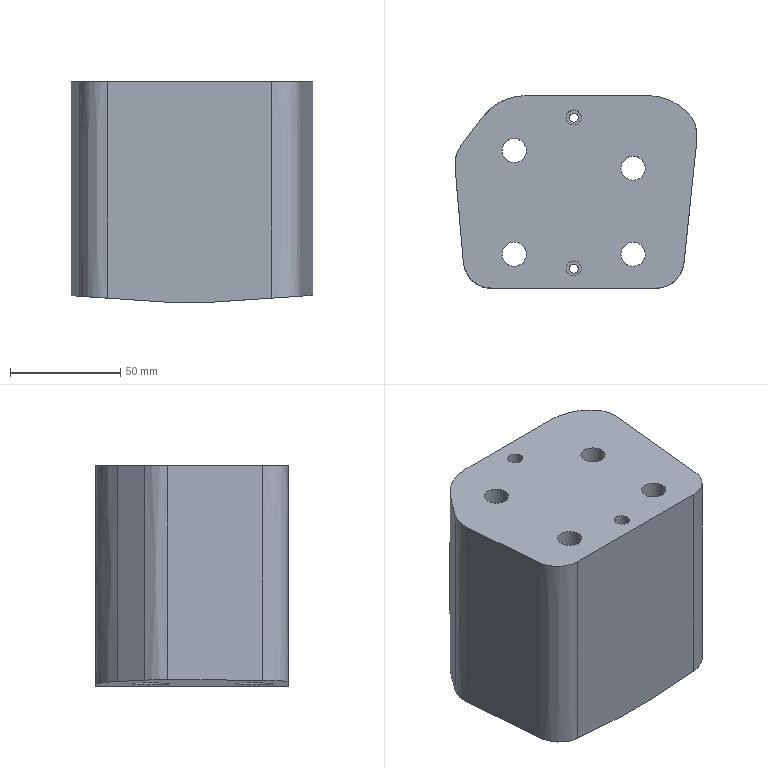Part | STEP file | lll_id3602_x_t | 1 solid | 42 faces | box 109.865 x 87.36 x 100 mm | volume 784681 mm3 | cylinder 18 | plane 18 | other 4 | cone 2 | commonest cylinder face diameters 11 x6 17 x4 4.1 x2 6.8 x2 8.506 x2 30 x1
STEP:
#1=CARTESIAN_POINT('',(3585.33,71.615,29.5));
#2=VERTEX_POINT('',#1);
#3=CARTESIAN_POINT('',(3587.38,71.615,29.5));
#4=DIRECTION('',(0.,0.,1.));
#5=DIRECTION('',(-1.,0.,0.));
#6=AXIS2_PLACEMENT_3D('',#3,#4,#5);
#7=CIRCLE('',#6,2.05);
#8=EDGE_CURVE('',#2,#2,#7,.T.);
#9=ORIENTED_EDGE('',*,*,#8,.T.);
#10=EDGE_LOOP('',(#9));
#11=FACE_BOUND('',#10,.T.);
#12=CARTESIAN_POINT('',(3587.38,73.665,-7.5));
#13=VERTEX_POINT('',#12);
#14=CARTESIAN_POINT('',(3587.38,71.615,-7.5));
#15=DIRECTION('',(0.,-0.000000008,1.));
#16=DIRECTION('',(0.,1.,0.000000008));
#17=AXIS2_PLACEMENT_3D('',#14,#15,#16);
#18=CIRCLE('',#17,2.05);
#19=EDGE_CURVE('',#13,#13,#18,.T.);
#20=ORIENTED_EDGE('',*,*,#19,.F.);
#21=EDGE_LOOP('',(#20));
#22=FACE_BOUND('',#21,.T.);
#23=CARTESIAN_POINT('',(3587.38,71.615,42.5));
#24=DIRECTION('',(0.,0.,-1.));
#25=DIRECTION('',(-0.0006834,1.,0.));
#26=AXIS2_PLACEMENT_3D('',#23,#24,#25);
#27=CYLINDRICAL_SURFACE('',#26,2.05);
#28=ADVANCED_FACE('',(#11,#22),#27,.F.);
#29=CARTESIAN_POINT('',(3585.326,140.05,29.5));
#30=VERTEX_POINT('',#29);
#31=CARTESIAN_POINT('',(3587.376,140.05,29.5));
#32=DIRECTION('',(0.,0.,1.));
#33=DIRECTION('',(-1.,0.,0.));
#34=AXIS2_PLACEMENT_3D('',#31,#32,#33);
#35=CIRCLE('',#34,2.05);
#36=EDGE_CURVE('',#30,#30,#35,.T.);
#37=ORIENTED_EDGE('',*,*,#36,.T.);
#38=EDGE_LOOP('',(#37));
#39=FACE_BOUND('',#38,.T.);
#40=CARTESIAN_POINT('',(3587.376,142.1,-7.5));
#41=VERTEX_POINT('',#40);
#42=CARTESIAN_POINT('',(3587.376,140.05,-7.5));
#43=DIRECTION('',(0.,-0.000000008,1.));
#44=DIRECTION('',(0.,1.,0.000000008));
#45=AXIS2_PLACEMENT_3D('',#42,#43,#44);
#46=CIRCLE('',#45,2.05);
#47=EDGE_CURVE('',#41,#41,#46,.T.);
#48=ORIENTED_EDGE('',*,*,#47,.F.);
#49=EDGE_LOOP('',(#48));
#50=FACE_BOUND('',#49,.T.);
#51=CARTESIAN_POINT('',(3587.376,140.05,42.5));
#52=DIRECTION('',(0.,0.,-1.));
#53=DIRECTION('',(0.,-1.,0.));
#54=AXIS2_PLACEMENT_3D('',#51,#52,#53);
#55=CYLINDRICAL_SURFACE('',#54,2.05);
#56=ADVANCED_FACE('',(#39,#50),#55,.F.);
#57=CARTESIAN_POINT('',(3614.279,69.531,62.5));
#58=VERTEX_POINT('',#57);
#59=CARTESIAN_POINT('',(3614.279,78.031,62.5));
#60=DIRECTION('',(0.,0.,-1.));
#61=DIRECTION('',(0.,-1.,0.));
#62=AXIS2_PLACEMENT_3D('',#59,#60,#61);
#63=CIRCLE('',#62,8.5);
#64=EDGE_CURVE('',#58,#58,#63,.T.);
#65=ORIENTED_EDGE('',*,*,#64,.F.);
#66=EDGE_LOOP('',(#65));
#67=FACE_BOUND('',#66,.T.);
#68=CARTESIAN_POINT('',(3622.779,78.031,-5.757));
#69=VERTEX_POINT('',#68);
#70=CARTESIAN_POINT('',(3614.279,78.031,-6.338));
#71=DIRECTION('',(0.06817,0.,-0.9977));
#72=DIRECTION('',(0.9977,0.,0.06817));
#73=AXIS2_PLACEMENT_3D('',#70,#71,#72);
#74=ELLIPSE('',#73,8.52,8.5);
#75=EDGE_CURVE('',#69,#69,#74,.T.);
#76=ORIENTED_EDGE('',*,*,#75,.T.);
#77=EDGE_LOOP('',(#76));
#78=FACE_BOUND('',#77,.T.);
#79=CARTESIAN_POINT('',(3614.279,78.031,12.5));
#80=DIRECTION('',(0.,0.,1.));
#81=DIRECTION('',(0.,1.,0.));
#82=AXIS2_PLACEMENT_3D('',#79,#80,#81);
#83=CYLINDRICAL_SURFACE('',#82,8.5);
#84=ADVANCED_FACE('',(#67,#78),#83,.F.);
#85=CARTESIAN_POINT('',(3638.507,142.694,92.5));
#86=VERTEX_POINT('',#85);
#87=CARTESIAN_POINT('',(3638.938,142.263,92.5));
#88=VERTEX_POINT('',#87);
#89=CARTESIAN_POINT('',(3565.868,215.334,92.5));
#90=DIRECTION('',(0.7071,-0.7071,0.));
#91=VECTOR('',#90,1.);
#92=LINE('',#89,#91);
#93=EDGE_CURVE('',#86,#88,#92,.T.);
#94=ORIENTED_EDGE('',*,*,#93,.T.);
#95=CARTESIAN_POINT('',(3638.938,142.263,-4.653));
#96=VERTEX_POINT('',#95);
#97=CARTESIAN_POINT('',(3638.938,142.263,0.00002208));
#98=DIRECTION('',(0.,0.000000008,-1.));
#99=VECTOR('',#98,1.);
#100=LINE('',#97,#99);
#101=EDGE_CURVE('',#88,#96,#100,.T.);
#102=ORIENTED_EDGE('',*,*,#101,.T.);
#103=CARTESIAN_POINT('',(3638.507,142.694,-4.682));
#104=VERTEX_POINT('',#103);
#105=CARTESIAN_POINT('',(3614.187,167.015,-6.344));
#106=DIRECTION('',(-0.7063,0.7063,-0.04826));
#107=VECTOR('',#106,1.);
#108=LINE('',#105,#107);
#109=EDGE_CURVE('',#96,#104,#108,.T.);
#110=ORIENTED_EDGE('',*,*,#109,.T.);
#111=CARTESIAN_POINT('',(3638.507,142.694,0.00002209));
#112=DIRECTION('',(0.,-0.000000008,1.));
#113=VECTOR('',#112,1.);
#114=LINE('',#111,#113);
#115=EDGE_CURVE('',#104,#86,#114,.T.);
#116=ORIENTED_EDGE('',*,*,#115,.T.);
#117=EDGE_LOOP('',(#94,#102,#110,#116));
#118=FACE_OUTER_BOUND('',#117,.T.);
#119=CARTESIAN_POINT('',(3638.507,142.694,0.00002209));
#120=DIRECTION('',(0.7071,0.7071,0.000000005));
#121=DIRECTION('',(0.7071,-0.7071,-0.000000005));
#122=AXIS2_PLACEMENT_3D('',#119,#120,#121);
#123=PLANE('',#122);
#124=ADVANCED_FACE('',(#118),#123,.T.);
#125=CARTESIAN_POINT('',(3577.268,62.657,-7.5));
#126=VERTEX_POINT('',#125);
#127=CARTESIAN_POINT('',(3550.037,62.657,-5.639));
#128=VERTEX_POINT('',#127);
#129=CARTESIAN_POINT('',(3586.78,62.657,-8.15));
#130=DIRECTION('',(-0.9977,-0.000000001,0.06817));
#131=VECTOR('',#130,1.);
#132=LINE('',#129,#131);
#133=EDGE_CURVE('',#126,#128,#132,.T.);
#134=ORIENTED_EDGE('',*,*,#133,.F.);
#135=CARTESIAN_POINT('',(3597.268,62.657,-7.5));
#136=VERTEX_POINT('',#135);
#137=CARTESIAN_POINT('',(3633.202,62.657,-7.5));
#138=DIRECTION('',(-1.,0.,0.));
#139=VECTOR('',#138,1.);
#140=LINE('',#137,#139);
#141=EDGE_CURVE('',#136,#126,#140,.T.);
#142=ORIENTED_EDGE('',*,*,#141,.F.);
#143=CARTESIAN_POINT('',(3624.637,62.657,-5.63));
#144=VERTEX_POINT('',#143);
#145=CARTESIAN_POINT('',(3597.268,62.657,-7.5));
#146=DIRECTION('',(-0.9977,0.,-0.06817));
#147=VECTOR('',#146,1.);
#148=LINE('',#145,#147);
#149=EDGE_CURVE('',#144,#136,#148,.T.);
#150=ORIENTED_EDGE('',*,*,#149,.F.);
#151=CARTESIAN_POINT('',(3624.637,62.657,92.5));
#152=VERTEX_POINT('',#151);
#153=CARTESIAN_POINT('',(3624.637,62.657,0.0000176));
#154=DIRECTION('',(0.,-0.000000008,1.));
#155=VECTOR('',#154,1.);
#156=LINE('',#153,#155);
#157=EDGE_CURVE('',#144,#152,#156,.T.);
#158=ORIENTED_EDGE('',*,*,#157,.T.);
#159=CARTESIAN_POINT('',(3550.037,62.657,92.5));
#160=VERTEX_POINT('',#159);
#161=CARTESIAN_POINT('',(3587.337,62.657,92.5));
#162=DIRECTION('',(-1.,0.,0.));
#163=VECTOR('',#162,1.);
#164=LINE('',#161,#163);
#165=EDGE_CURVE('',#152,#160,#164,.T.);
#166=ORIENTED_EDGE('',*,*,#165,.T.);
#167=CARTESIAN_POINT('',(3550.037,62.657,0.0000176));
#168=DIRECTION('',(0.,-0.000000008,1.));
#169=VECTOR('',#168,1.);
#170=LINE('',#167,#169);
#171=EDGE_CURVE('',#128,#160,#170,.T.);
#172=ORIENTED_EDGE('',*,*,#171,.F.);
#173=EDGE_LOOP('',(#134,#142,#150,#158,#166,#172));
#174=FACE_OUTER_BOUND('',#173,.T.);
#175=CARTESIAN_POINT('',(3587.337,62.657,0.0000176));
#176=DIRECTION('',(0.,1.,0.000000008));
#177=DIRECTION('',(-1.,0.,0.));
#178=AXIS2_PLACEMENT_3D('',#175,#176,#177);
#179=PLANE('',#178);
#180=ADVANCED_FACE('',(#174),#179,.F.);
#181=ORIENTED_EDGE('',*,*,#157,.F.);
#182=CARTESIAN_POINT('',(3637.367,74.119,-4.76));
#183=VERTEX_POINT('',#182);
#184=CARTESIAN_POINT('',(3624.637,62.657,-5.63));
#185=CARTESIAN_POINT('',(3627.788,62.657,-5.415));
#186=CARTESIAN_POINT('',(3630.864,63.843,-5.204));
#187=CARTESIAN_POINT('',(3635.521,68.029,-4.886));
#188=CARTESIAN_POINT('',(3637.037,70.974,-4.783));
#189=CARTESIAN_POINT('',(3637.367,74.119,-4.76));
#190=B_SPLINE_CURVE_WITH_KNOTS('',3,(#184,#185,#186,#187,#188,#189),.UNSPECIFIED.,.F.,.F.,(4,2,4),(0.,0.5,1.),.UNSPECIFIED.);
#191=EDGE_CURVE('',#144,#183,#190,.T.);
#192=ORIENTED_EDGE('',*,*,#191,.T.);
#193=CARTESIAN_POINT('',(3637.367,74.119,92.5));
#194=VERTEX_POINT('',#193);
#195=CARTESIAN_POINT('',(3637.367,74.119,0.00001769));
#196=DIRECTION('',(0.,-0.000000008,1.));
#197=VECTOR('',#196,1.);
#198=LINE('',#195,#197);
#199=EDGE_CURVE('',#183,#194,#198,.T.);
#200=ORIENTED_EDGE('',*,*,#199,.T.);
#201=CARTESIAN_POINT('',(3637.367,74.119,92.5));
#202=CARTESIAN_POINT('',(3637.037,70.982,92.5));
#203=CARTESIAN_POINT('',(3635.532,68.044,92.5));
#204=CARTESIAN_POINT('',(3630.881,63.852,92.5));
#205=CARTESIAN_POINT('',(3627.795,62.657,92.5));
#206=CARTESIAN_POINT('',(3624.637,62.657,92.5));
#207=B_SPLINE_CURVE_WITH_KNOTS('',3,(#201,#202,#203,#204,#205,#206),.UNSPECIFIED.,.F.,.F.,(4,2,4),(0.,0.5,1.),.UNSPECIFIED.);
#208=EDGE_CURVE('',#194,#152,#207,.T.);
#209=ORIENTED_EDGE('',*,*,#208,.T.);
#210=EDGE_LOOP('',(#181,#192,#200,#209));
#211=FACE_OUTER_BOUND('',#210,.T.);
#212=CARTESIAN_POINT('',(3637.367,74.119,0.00001769));
#213=CARTESIAN_POINT('',(3637.202,72.546,0.00001768));
#214=CARTESIAN_POINT('',(3636.76,71.054,0.00001767));
#215=CARTESIAN_POINT('',(3635.324,68.237,0.00001764));
#216=CARTESIAN_POINT('',(3634.377,67.002,0.00001763));
#217=CARTESIAN_POINT('',(3632.027,64.886,0.00001762));
#218=CARTESIAN_POINT('',(3630.701,64.074,0.00001761));
#219=CARTESIAN_POINT('',(3627.748,62.94,0.0000176));
#220=CARTESIAN_POINT('',(3626.219,62.657,0.0000176));
#221=CARTESIAN_POINT('',(3624.637,62.657,0.0000176));
#222=B_SPLINE_CURVE_WITH_KNOTS('',3,(#212,#213,#214,#215,#216,#217,#218,#219,#220,#221),.UNSPECIFIED.,.F.,.F.,(4,2,2,2,4),(0.,0.25,0.5,0.75,1.),.UNSPECIFIED.);
#223=DIRECTION('',(0.,-0.000000008,1.));
#224=VECTOR('',#223,1.);
#225=SURFACE_OF_LINEAR_EXTRUSION('',#222,#224);
#226=ADVANCED_FACE('',(#211),#225,.F.);
#227=CARTESIAN_POINT('',(3643.25,130.089,-4.358));
#228=VERTEX_POINT('',#227);
#229=CARTESIAN_POINT('',(3639.156,91.137,-4.638));
#230=DIRECTION('',(0.1045,0.9945,0.007142));
#231=VECTOR('',#230,1.);
#232=LINE('',#229,#231);
#233=EDGE_CURVE('',#183,#228,#232,.T.);
#234=ORIENTED_EDGE('',*,*,#233,.T.);
#235=CARTESIAN_POINT('',(3643.25,130.089,92.5));
#236=VERTEX_POINT('',#235);
#237=CARTESIAN_POINT('',(3643.25,130.089,0.00001811));
#238=DIRECTION('',(0.,-0.000000008,1.));
#239=VECTOR('',#238,1.);
#240=LINE('',#237,#239);
#241=EDGE_CURVE('',#228,#236,#240,.T.);
#242=ORIENTED_EDGE('',*,*,#241,.T.);
#243=CARTESIAN_POINT('',(3639.152,91.104,92.5));
#244=DIRECTION('',(-0.1045,-0.9945,0.));
#245=VECTOR('',#244,1.);
#246=LINE('',#243,#245);
#247=EDGE_CURVE('',#236,#194,#246,.T.);
#248=ORIENTED_EDGE('',*,*,#247,.T.);
#249=ORIENTED_EDGE('',*,*,#199,.F.);
#250=EDGE_LOOP('',(#234,#242,#248,#249));
#251=FACE_OUTER_BOUND('',#250,.T.);
#252=CARTESIAN_POINT('',(3639.152,91.104,0.00001782));
#253=DIRECTION('',(-0.9945,0.1045,0.000000001));
#254=DIRECTION('',(-0.1045,-0.9945,-0.000000008));
#255=AXIS2_PLACEMENT_3D('',#252,#253,#254);
#256=PLANE('',#255);
#257=ADVANCED_FACE('',(#251),#256,.F.);
#258=CARTESIAN_POINT('',(3614.279,108.531,62.5));
#259=VERTEX_POINT('',#258);
#260=CARTESIAN_POINT('',(3614.279,117.031,62.5));
#261=DIRECTION('',(0.,0.,-1.));
#262=DIRECTION('',(0.,-1.,0.));
#263=AXIS2_PLACEMENT_3D('',#260,#261,#262);
#264=CIRCLE('',#263,8.5);
#265=EDGE_CURVE('',#259,#259,#264,.T.);
#266=ORIENTED_EDGE('',*,*,#265,.F.);
#267=EDGE_LOOP('',(#266));
#268=FACE_BOUND('',#267,.T.);
#269=CARTESIAN_POINT('',(3622.779,117.031,-5.757));
#270=VERTEX_POINT('',#269);
#271=CARTESIAN_POINT('',(3614.279,117.031,-6.338));
#272=DIRECTION('',(-0.06817,0.,0.9977));
#273=DIRECTION('',(0.9977,0.,0.06817));
#274=AXIS2_PLACEMENT_3D('',#271,#272,#273);
#275=ELLIPSE('',#274,8.52,8.5);
#276=EDGE_CURVE('',#270,#270,#275,.T.);
#277=ORIENTED_EDGE('',*,*,#276,.F.);
#278=EDGE_LOOP('',(#277));
#279=FACE_BOUND('',#278,.T.);
#280=CARTESIAN_POINT('',(3614.279,117.031,12.5));
#281=DIRECTION('',(0.,0.,1.));
#282=DIRECTION('',(0.,1.,0.));
#283=AXIS2_PLACEMENT_3D('',#280,#281,#282);
#284=CYLINDRICAL_SURFACE('',#283,8.5);
#285=ADVANCED_FACE('',(#268,#279),#284,.F.);
#286=ORIENTED_EDGE('',*,*,#47,.T.);
#287=EDGE_LOOP('',(#286));
#288=FACE_BOUND('',#287,.T.);
#289=ORIENTED_EDGE('',*,*,#19,.T.);
#290=EDGE_LOOP('',(#289));
#291=FACE_BOUND('',#290,.T.);
#292=CARTESIAN_POINT('',(3587.38,92.115,-7.5));
#293=VERTEX_POINT('',#292);
#294=CARTESIAN_POINT('',(3587.38,86.615,-7.5));
#295=DIRECTION('',(0.,-0.000000008,1.));
#296=DIRECTION('',(0.,1.,0.000000008));
#297=AXIS2_PLACEMENT_3D('',#294,#295,#296);
#298=CIRCLE('',#297,5.5);
#299=EDGE_CURVE('',#293,#293,#298,.T.);
#300=ORIENTED_EDGE('',*,*,#299,.T.);
#301=EDGE_LOOP('',(#300));
#302=FACE_BOUND('',#301,.T.);
#303=CARTESIAN_POINT('',(3587.38,130.115,-7.5));
#304=VERTEX_POINT('',#303);
#305=CARTESIAN_POINT('',(3587.38,124.615,-7.5));
#306=DIRECTION('',(0.,-0.000000008,1.));
#307=DIRECTION('',(0.,1.,0.000000008));
#308=AXIS2_PLACEMENT_3D('',#305,#306,#307);
#309=CIRCLE('',#308,5.5);
#310=EDGE_CURVE('',#304,#304,#309,.T.);
#311=ORIENTED_EDGE('',*,*,#310,.T.);
#312=EDGE_LOOP('',(#311));
#313=FACE_BOUND('',#312,.T.);
#314=ORIENTED_EDGE('',*,*,#141,.T.);
#315=CARTESIAN_POINT('',(3577.268,150.017,-7.5));
#316=VERTEX_POINT('',#315);
#317=CARTESIAN_POINT('',(3577.268,65.944,-7.5));
#318=DIRECTION('',(-0.000000111,1.,0.000000008));
#319=VECTOR('',#318,1.);
#320=LINE('',#317,#319);
#321=EDGE_CURVE('',#126,#316,#320,.T.);
#322=ORIENTED_EDGE('',*,*,#321,.T.);
#323=CARTESIAN_POINT('',(3597.268,150.017,-7.5));
#324=VERTEX_POINT('',#323);
#325=CARTESIAN_POINT('',(3633.202,150.017,-7.5));
#326=DIRECTION('',(1.,0.,0.));
#327=VECTOR('',#326,1.);
#328=LINE('',#325,#327);
#329=EDGE_CURVE('',#316,#324,#328,.T.);
#330=ORIENTED_EDGE('',*,*,#329,.T.);
#331=CARTESIAN_POINT('',(3597.268,62.657,-7.5));
#332=DIRECTION('',(0.,1.,0.));
#333=VECTOR('',#332,1.);
#334=LINE('',#331,#333);
#335=EDGE_CURVE('',#136,#324,#334,.T.);
#336=ORIENTED_EDGE('',*,*,#335,.F.);
#337=EDGE_LOOP('',(#314,#322,#330,#336));
#338=FACE_BOUND('',#337,.T.);
#339=CARTESIAN_POINT('',(3633.202,65.944,-7.5));
#340=DIRECTION('',(0.,-0.000000008,1.));
#341=DIRECTION('',(0.,1.,0.000000008));
#342=AXIS2_PLACEMENT_3D('',#339,#340,#341);
#343=PLANE('',#342);
#344=ADVANCED_FACE('',(#288,#291,#302,#313,#338),#343,.F.);
#345=ORIENTED_EDGE('',*,*,#64,.T.);
#346=EDGE_LOOP('',(#345));
#347=FACE_BOUND('',#346,.T.);
#348=CARTESIAN_POINT('',(3608.779,78.031,62.5));
#349=VERTEX_POINT('',#348);
#350=CARTESIAN_POINT('',(3614.279,78.031,62.5));
#351=DIRECTION('',(0.,0.,-1.));
#352=DIRECTION('',(-1.,0.,0.));
#353=AXIS2_PLACEMENT_3D('',#350,#351,#352);
#354=CIRCLE('',#353,5.5);
#355=EDGE_CURVE('',#349,#349,#354,.T.);
#356=ORIENTED_EDGE('',*,*,#355,.F.);
#357=EDGE_LOOP('',(#356));
#358=FACE_BOUND('',#357,.T.);
#359=CARTESIAN_POINT('',(3614.279,78.031,62.5));
#360=DIRECTION('',(0.,0.,1.));
#361=DIRECTION('',(0.,1.,0.));
#362=AXIS2_PLACEMENT_3D('',#359,#360,#361);
#363=PLANE('',#362);
#364=ADVANCED_FACE('',(#347,#358),#363,.F.);
#365=CARTESIAN_POINT('',(3560.376,69.55,62.5));
#366=VERTEX_POINT('',#365);
#367=CARTESIAN_POINT('',(3560.376,78.05,62.5));
#368=DIRECTION('',(0.,0.,-1.));
#369=DIRECTION('',(0.,-1.,0.));
#370=AXIS2_PLACEMENT_3D('',#367,#368,#369);
#371=CIRCLE('',#370,8.5);
#372=EDGE_CURVE('',#366,#366,#371,.T.);
#373=ORIENTED_EDGE('',*,*,#372,.T.);
#374=EDGE_LOOP('',(#373));
#375=FACE_BOUND('',#374,.T.);
#376=CARTESIAN_POINT('',(3554.876,78.05,62.5));
#377=VERTEX_POINT('',#376);
#378=CARTESIAN_POINT('',(3560.376,78.05,62.5));
#379=DIRECTION('',(0.,0.,-1.));
#380=DIRECTION('',(-1.,0.,0.));
#381=AXIS2_PLACEMENT_3D('',#378,#379,#380);
#382=CIRCLE('',#381,5.5);
#383=EDGE_CURVE('',#377,#377,#382,.T.);
#384=ORIENTED_EDGE('',*,*,#383,.F.);
#385=EDGE_LOOP('',(#384));
#386=FACE_BOUND('',#385,.T.);
#387=CARTESIAN_POINT('',(3560.376,78.05,62.5));
#388=DIRECTION('',(0.,0.,1.));
#389=DIRECTION('',(0.,1.,0.));
#390=AXIS2_PLACEMENT_3D('',#387,#388,#389);
#391=PLANE('',#390);
#392=ADVANCED_FACE('',(#375,#386),#391,.F.);
#393=ORIENTED_EDGE('',*,*,#265,.T.);
#394=EDGE_LOOP('',(#393));
#395=FACE_BOUND('',#394,.T.);
#396=CARTESIAN_POINT('',(3608.779,117.031,62.5));
#397=VERTEX_POINT('',#396);
#398=CARTESIAN_POINT('',(3614.279,117.031,62.5));
#399=DIRECTION('',(0.,0.,-1.));
#400=DIRECTION('',(-1.,0.,0.));
#401=AXIS2_PLACEMENT_3D('',#398,#399,#400);
#402=CIRCLE('',#401,5.5);
#403=EDGE_CURVE('',#397,#397,#402,.T.);
#404=ORIENTED_EDGE('',*,*,#403,.F.);
#405=EDGE_LOOP('',(#404));
#406=FACE_BOUND('',#405,.T.);
#407=CARTESIAN_POINT('',(3614.279,117.031,62.5));
#408=DIRECTION('',(0.,0.,1.));
#409=DIRECTION('',(0.,1.,0.));
#410=AXIS2_PLACEMENT_3D('',#407,#408,#409);
#411=PLANE('',#410);
#412=ADVANCED_FACE('',(#395,#406),#411,.F.);
#413=CARTESIAN_POINT('',(3560.376,116.55,62.5));
#414=VERTEX_POINT('',#413);
#415=CARTESIAN_POINT('',(3560.376,125.05,62.5));
#416=DIRECTION('',(0.,0.,-1.));
#417=DIRECTION('',(0.,-1.,0.));
#418=AXIS2_PLACEMENT_3D('',#415,#416,#417);
#419=CIRCLE('',#418,8.5);
#420=EDGE_CURVE('',#414,#414,#419,.T.);
#421=ORIENTED_EDGE('',*,*,#420,.T.);
#422=EDGE_LOOP('',(#421));
#423=FACE_BOUND('',#422,.T.);
#424=CARTESIAN_POINT('',(3554.876,125.05,62.5));
#425=VERTEX_POINT('',#424);
#426=CARTESIAN_POINT('',(3560.376,125.05,62.5));
#427=DIRECTION('',(0.,0.,-1.));
#428=DIRECTION('',(-1.,0.,0.));
#429=AXIS2_PLACEMENT_3D('',#426,#427,#428);
#430=CIRCLE('',#429,5.5);
#431=EDGE_CURVE('',#425,#425,#430,.T.);
#432=ORIENTED_EDGE('',*,*,#431,.F.);
#433=EDGE_LOOP('',(#432));
#434=FACE_BOUND('',#433,.T.);
#435=CARTESIAN_POINT('',(3560.376,125.05,62.5));
#436=DIRECTION('',(0.,0.,1.));
#437=DIRECTION('',(0.,1.,0.));
#438=AXIS2_PLACEMENT_3D('',#435,#436,#437);
#439=PLANE('',#438);
#440=ADVANCED_FACE('',(#423,#434),#439,.F.);
#441=CARTESIAN_POINT('',(3587.378,75.015,92.5));
#442=VERTEX_POINT('',#441);
#443=CARTESIAN_POINT('',(3587.38,71.615,92.5));
#444=DIRECTION('',(0.,0.,1.));
#445=DIRECTION('',(-0.0006834,1.,0.));
#446=AXIS2_PLACEMENT_3D('',#443,#444,#445);
#447=CIRCLE('',#446,3.4);
#448=EDGE_CURVE('',#442,#442,#447,.T.);
#449=ORIENTED_EDGE('',*,*,#448,.T.);
#450=EDGE_LOOP('',(#449));
#451=FACE_BOUND('',#450,.T.);
#452=CARTESIAN_POINT('',(3587.382,68.215,29.5));
#453=VERTEX_POINT('',#452);
#454=CARTESIAN_POINT('',(3587.38,71.615,29.5));
#455=DIRECTION('',(0.,0.,1.));
#456=DIRECTION('',(0.0006834,-1.,0.));
#457=AXIS2_PLACEMENT_3D('',#454,#455,#456);
#458=CIRCLE('',#457,3.4);
#459=EDGE_CURVE('',#453,#453,#458,.T.);
#460=ORIENTED_EDGE('',*,*,#459,.F.);
#461=EDGE_LOOP('',(#460));
#462=FACE_BOUND('',#461,.T.);
#463=CARTESIAN_POINT('',(3587.38,71.615,42.5));
#464=DIRECTION('',(0.,0.,1.));
#465=DIRECTION('',(0.0006834,-1.,0.));
#466=AXIS2_PLACEMENT_3D('',#463,#464,#465);
#467=CYLINDRICAL_SURFACE('',#466,3.4);
#468=ADVANCED_FACE('',(#451,#462),#467,.F.);
#469=CARTESIAN_POINT('',(3565.78,150.017,92.5));
#470=VERTEX_POINT('',#469);
#471=CARTESIAN_POINT('',(3620.83,150.017,92.5));
#472=VERTEX_POINT('',#471);
#473=CARTESIAN_POINT('',(3581.149,150.017,92.5));
#474=DIRECTION('',(1.,0.,0.));
#475=VECTOR('',#474,1.);
#476=LINE('',#473,#475);
#477=EDGE_CURVE('',#470,#472,#476,.T.);
#478=ORIENTED_EDGE('',*,*,#477,.T.);
#479=CARTESIAN_POINT('',(3620.83,150.017,-5.89));
#480=VERTEX_POINT('',#479);
#481=CARTESIAN_POINT('',(3620.83,150.017,0.00001826));
#482=DIRECTION('',(0.,0.000000008,-1.));
#483=VECTOR('',#482,1.);
#484=LINE('',#481,#483);
#485=EDGE_CURVE('',#472,#480,#484,.T.);
#486=ORIENTED_EDGE('',*,*,#485,.T.);
#487=CARTESIAN_POINT('',(3581.734,150.017,-8.561));
#488=DIRECTION('',(0.9977,-0.000000001,0.06817));
#489=VECTOR('',#488,1.);
#490=LINE('',#487,#489);
#491=EDGE_CURVE('',#324,#480,#490,.T.);
#492=ORIENTED_EDGE('',*,*,#491,.F.);
#493=ORIENTED_EDGE('',*,*,#329,.F.);
#494=CARTESIAN_POINT('',(3565.78,150.017,-6.715));
#495=VERTEX_POINT('',#494);
#496=CARTESIAN_POINT('',(3580.621,150.017,-7.729));
#497=DIRECTION('',(0.9977,0.000000001,-0.06817));
#498=VECTOR('',#497,1.);
#499=LINE('',#496,#498);
#500=EDGE_CURVE('',#495,#316,#499,.T.);
#501=ORIENTED_EDGE('',*,*,#500,.F.);
#502=CARTESIAN_POINT('',(3565.78,150.017,0.00001826));
#503=DIRECTION('',(0.,-0.000000008,1.));
#504=VECTOR('',#503,1.);
#505=LINE('',#502,#504);
#506=EDGE_CURVE('',#495,#470,#505,.T.);
#507=ORIENTED_EDGE('',*,*,#506,.T.);
#508=EDGE_LOOP('',(#478,#486,#492,#493,#501,#507));
#509=FACE_OUTER_BOUND('',#508,.T.);
#510=CARTESIAN_POINT('',(3581.149,150.017,0.00001826));
#511=DIRECTION('',(0.,-1.,-0.000000008));
#512=DIRECTION('',(1.,0.,0.));
#513=AXIS2_PLACEMENT_3D('',#510,#511,#512);
#514=PLANE('',#513);
#515=ADVANCED_FACE('',(#509),#514,.F.);
#516=CARTESIAN_POINT('',(3545.814,140.062,-5.351));
#517=VERTEX_POINT('',#516);
#518=CARTESIAN_POINT('',(3545.814,140.062,-5.351));
#519=CARTESIAN_POINT('',(3548.156,143.17,-5.511));
#520=CARTESIAN_POINT('',(3551.205,145.688,-5.719));
#521=CARTESIAN_POINT('',(3556.361,148.254,-6.071));
#522=CARTESIAN_POINT('',(3558.204,148.928,-6.197));
#523=CARTESIAN_POINT('',(3561.934,149.802,-6.452));
#524=CARTESIAN_POINT('',(3563.838,150.017,-6.582));
#525=CARTESIAN_POINT('',(3565.78,150.017,-6.715));
#526=B_SPLINE_CURVE_WITH_KNOTS('',3,(#518,#519,#520,#521,#522,#523,#524,#525),.UNSPECIFIED.,.F.,.F.,(4,2,2,4),(0.,0.5,0.75,1.),.UNSPECIFIED.);
#527=EDGE_CURVE('',#517,#495,#526,.T.);
#528=ORIENTED_EDGE('',*,*,#527,.F.);
#529=CARTESIAN_POINT('',(3545.814,140.062,92.5));
#530=VERTEX_POINT('',#529);
#531=CARTESIAN_POINT('',(3545.814,140.062,0.00001819));
#532=DIRECTION('',(0.,-0.000000008,1.));
#533=VECTOR('',#532,1.);
#534=LINE('',#531,#533);
#535=EDGE_CURVE('',#517,#530,#534,.T.);
#536=ORIENTED_EDGE('',*,*,#535,.T.);
#537=CARTESIAN_POINT('',(3545.814,140.062,92.5));
#538=CARTESIAN_POINT('',(3548.154,143.168,92.5));
#539=CARTESIAN_POINT('',(3551.201,145.685,92.5));
#540=CARTESIAN_POINT('',(3556.357,148.252,92.5));
#541=CARTESIAN_POINT('',(3558.2,148.927,92.5));
#542=CARTESIAN_POINT('',(3561.932,149.802,92.5));
#543=CARTESIAN_POINT('',(3563.837,150.017,92.5));
#544=CARTESIAN_POINT('',(3565.78,150.017,92.5));
#545=B_SPLINE_CURVE_WITH_KNOTS('',3,(#537,#538,#539,#540,#541,#542,#543,#544),.UNSPECIFIED.,.F.,.F.,(4,2,2,4),(0.,0.5,0.75,1.),.UNSPECIFIED.);
#546=EDGE_CURVE('',#530,#470,#545,.T.);
#547=ORIENTED_EDGE('',*,*,#546,.T.);
#548=ORIENTED_EDGE('',*,*,#506,.F.);
#549=EDGE_LOOP('',(#528,#536,#547,#548));
#550=FACE_OUTER_BOUND('',#549,.T.);
#551=CARTESIAN_POINT('',(3545.814,140.062,0.00001819));
#552=CARTESIAN_POINT('',(3548.176,143.196,0.00001821));
#553=CARTESIAN_POINT('',(3551.113,145.639,0.00001823));
#554=CARTESIAN_POINT('',(3558.137,149.141,0.00001826));
#555=CARTESIAN_POINT('',(3561.855,150.017,0.00001826));
#556=CARTESIAN_POINT('',(3565.78,150.017,0.00001826));
#557=B_SPLINE_CURVE_WITH_KNOTS('',3,(#551,#552,#553,#554,#555,#556),.UNSPECIFIED.,.F.,.F.,(4,2,4),(0.,0.5,1.),.UNSPECIFIED.);
#558=DIRECTION('',(0.,-0.000000008,1.));
#559=VECTOR('',#558,1.);
#560=SURFACE_OF_LINEAR_EXTRUSION('',#557,#559);
#561=ADVANCED_FACE('',(#550),#560,.F.);
#562=CARTESIAN_POINT('',(3536.487,127.684,-4.713));
#563=VERTEX_POINT('',#562);
#564=CARTESIAN_POINT('',(3541.026,133.708,-5.024));
#565=DIRECTION('',(-0.6013,-0.798,0.04109));
#566=VECTOR('',#565,1.);
#567=LINE('',#564,#566);
#568=EDGE_CURVE('',#517,#563,#567,.T.);
#569=ORIENTED_EDGE('',*,*,#568,.T.);
#570=CARTESIAN_POINT('',(3536.487,127.684,92.5));
#571=VERTEX_POINT('',#570);
#572=CARTESIAN_POINT('',(3536.487,127.684,0.00001809));
#573=DIRECTION('',(0.,-0.000000008,1.));
#574=VECTOR('',#573,1.);
#575=LINE('',#572,#574);
#576=EDGE_CURVE('',#563,#571,#575,.T.);
#577=ORIENTED_EDGE('',*,*,#576,.T.);
#578=CARTESIAN_POINT('',(3541.15,133.873,92.5));
#579=DIRECTION('',(0.6018,0.7986,0.));
#580=VECTOR('',#579,1.);
#581=LINE('',#578,#580);
#582=EDGE_CURVE('',#571,#530,#581,.T.);
#583=ORIENTED_EDGE('',*,*,#582,.T.);
#584=ORIENTED_EDGE('',*,*,#535,.F.);
#585=EDGE_LOOP('',(#569,#577,#583,#584));
#586=FACE_OUTER_BOUND('',#585,.T.);
#587=CARTESIAN_POINT('',(3541.15,133.873,0.00001814));
#588=DIRECTION('',(0.7986,-0.6018,-0.000000005));
#589=DIRECTION('',(0.6018,0.7986,0.000000006));
#590=AXIS2_PLACEMENT_3D('',#587,#588,#589);
#591=PLANE('',#590);
#592=ADVANCED_FACE('',(#586),#591,.F.);
#593=CARTESIAN_POINT('',(3533.523,117.349,-4.511));
#594=VERTEX_POINT('',#593);
#595=CARTESIAN_POINT('',(3536.487,127.684,-4.713));
#596=CARTESIAN_POINT('',(3534.268,124.74,-4.562));
#597=CARTESIAN_POINT('',(3533.202,121.024,-4.489));
#598=CARTESIAN_POINT('',(3533.523,117.349,-4.511));
#599=B_SPLINE_CURVE_WITH_KNOTS('',3,(#595,#596,#597,#598),.UNSPECIFIED.,.F.,.F.,(4,4),(0.,1.),.UNSPECIFIED.);
#600=EDGE_CURVE('',#563,#594,#599,.T.);
#601=ORIENTED_EDGE('',*,*,#600,.T.);
#602=CARTESIAN_POINT('',(3533.523,117.349,92.5));
#603=VERTEX_POINT('',#602);
#604=CARTESIAN_POINT('',(3533.523,117.349,0.00001802));
#605=DIRECTION('',(0.,-0.000000008,1.));
#606=VECTOR('',#605,1.);
#607=LINE('',#604,#606);
#608=EDGE_CURVE('',#594,#603,#607,.T.);
#609=ORIENTED_EDGE('',*,*,#608,.T.);
#610=CARTESIAN_POINT('',(3533.523,117.349,92.5));
#611=CARTESIAN_POINT('',(3533.202,121.023,92.5));
#612=CARTESIAN_POINT('',(3534.267,124.739,92.5));
#613=CARTESIAN_POINT('',(3536.487,127.684,92.5));
#614=B_SPLINE_CURVE_WITH_KNOTS('',3,(#610,#611,#612,#613),.UNSPECIFIED.,.F.,.F.,(4,4),(0.,1.),.UNSPECIFIED.);
#615=EDGE_CURVE('',#603,#571,#614,.T.);
#616=ORIENTED_EDGE('',*,*,#615,.T.);
#617=ORIENTED_EDGE('',*,*,#576,.F.);
#618=EDGE_LOOP('',(#601,#609,#616,#617));
#619=FACE_OUTER_BOUND('',#618,.T.);
#620=CARTESIAN_POINT('',(3533.523,117.349,0.00001802));
#621=CARTESIAN_POINT('',(3533.362,119.195,0.00001803));
#622=CARTESIAN_POINT('',(3533.536,121.01,0.00001804));
#623=CARTESIAN_POINT('',(3534.558,124.573,0.00001807));
#624=CARTESIAN_POINT('',(3535.371,126.204,0.00001808));
#625=CARTESIAN_POINT('',(3536.487,127.684,0.00001809));
#626=B_SPLINE_CURVE_WITH_KNOTS('',3,(#620,#621,#622,#623,#624,#625),.UNSPECIFIED.,.F.,.F.,(4,2,4),(0.,0.5,1.),.UNSPECIFIED.);
#627=DIRECTION('',(0.,-0.000000008,1.));
#628=VECTOR('',#627,1.);
#629=SURFACE_OF_LINEAR_EXTRUSION('',#626,#628);
#630=ADVANCED_FACE('',(#619),#629,.F.);
#631=CARTESIAN_POINT('',(3537.286,74.341,-4.768));
#632=VERTEX_POINT('',#631);
#633=CARTESIAN_POINT('',(3535.402,95.873,-4.639));
#634=DIRECTION('',(-0.08715,0.9962,0.005955));
#635=VECTOR('',#634,1.);
#636=LINE('',#633,#635);
#637=EDGE_CURVE('',#632,#594,#636,.T.);
#638=ORIENTED_EDGE('',*,*,#637,.F.);
#639=CARTESIAN_POINT('',(3537.286,74.341,92.5));
#640=VERTEX_POINT('',#639);
#641=CARTESIAN_POINT('',(3537.286,74.341,0.00001769));
#642=DIRECTION('',(0.,-0.000000008,1.));
#643=VECTOR('',#642,1.);
#644=LINE('',#641,#643);
#645=EDGE_CURVE('',#632,#640,#644,.T.);
#646=ORIENTED_EDGE('',*,*,#645,.T.);
#647=CARTESIAN_POINT('',(3535.404,95.845,92.5));
#648=DIRECTION('',(-0.08716,0.9962,0.));
#649=VECTOR('',#648,1.);
#650=LINE('',#647,#649);
#651=EDGE_CURVE('',#640,#603,#650,.T.);
#652=ORIENTED_EDGE('',*,*,#651,.T.);
#653=ORIENTED_EDGE('',*,*,#608,.F.);
#654=EDGE_LOOP('',(#638,#646,#652,#653));
#655=FACE_OUTER_BOUND('',#654,.T.);
#656=CARTESIAN_POINT('',(3535.404,95.845,0.00001785));
#657=DIRECTION('',(0.9962,0.08716,0.000000001));
#658=DIRECTION('',(-0.08716,0.9962,0.000000008));
#659=AXIS2_PLACEMENT_3D('',#656,#657,#658);
#660=PLANE('',#659);
#661=ADVANCED_FACE('',(#655),#660,.F.);
#662=CARTESIAN_POINT('',(3537.286,74.341,-4.768));
#663=CARTESIAN_POINT('',(3537.564,71.158,-4.787));
#664=CARTESIAN_POINT('',(3539.056,68.157,-4.889));
#665=CARTESIAN_POINT('',(3543.723,63.882,-5.208));
#666=CARTESIAN_POINT('',(3546.846,62.657,-5.421));
#667=CARTESIAN_POINT('',(3550.037,62.657,-5.639));
#668=B_SPLINE_CURVE_WITH_KNOTS('',3,(#662,#663,#664,#665,#666,#667),.UNSPECIFIED.,.F.,.F.,(4,2,4),(0.,0.5,1.),.UNSPECIFIED.);
#669=EDGE_CURVE('',#632,#128,#668,.T.);
#670=ORIENTED_EDGE('',*,*,#669,.T.);
#671=ORIENTED_EDGE('',*,*,#171,.T.);
#672=CARTESIAN_POINT('',(3550.037,62.657,92.5));
#673=CARTESIAN_POINT('',(3546.846,62.657,92.5));
#674=CARTESIAN_POINT('',(3543.729,63.878,92.5));
#675=CARTESIAN_POINT('',(3539.06,68.152,92.5));
#676=CARTESIAN_POINT('',(3537.564,71.158,92.5));
#677=CARTESIAN_POINT('',(3537.286,74.341,92.5));
#678=B_SPLINE_CURVE_WITH_KNOTS('',3,(#672,#673,#674,#675,#676,#677),.UNSPECIFIED.,.F.,.F.,(4,2,4),(0.,0.5,1.),.UNSPECIFIED.);
#679=EDGE_CURVE('',#160,#640,#678,.T.);
#680=ORIENTED_EDGE('',*,*,#679,.T.);
#681=ORIENTED_EDGE('',*,*,#645,.F.);
#682=EDGE_LOOP('',(#670,#671,#680,#681));
#683=FACE_OUTER_BOUND('',#682,.T.);
#684=CARTESIAN_POINT('',(3550.037,62.657,0.0000176));
#685=CARTESIAN_POINT('',(3548.437,62.657,0.0000176));
#686=CARTESIAN_POINT('',(3546.89,62.947,0.0000176));
#687=CARTESIAN_POINT('',(3543.906,64.107,0.00001761));
#688=CARTESIAN_POINT('',(3542.57,64.938,0.00001762));
#689=CARTESIAN_POINT('',(3540.21,67.101,0.00001764));
#690=CARTESIAN_POINT('',(3539.265,68.36,0.00001765));
#691=CARTESIAN_POINT('',(3537.849,71.231,0.00001767));
#692=CARTESIAN_POINT('',(3537.425,72.746,0.00001768));
#693=CARTESIAN_POINT('',(3537.286,74.341,0.00001769));
#694=B_SPLINE_CURVE_WITH_KNOTS('',3,(#684,#685,#686,#687,#688,#689,#690,#691,#692,#693),.UNSPECIFIED.,.F.,.F.,(4,2,2,2,4),(0.,0.25,0.5,0.75,1.),.UNSPECIFIED.);
#695=DIRECTION('',(0.,-0.000000008,1.));
#696=VECTOR('',#695,1.);
#697=SURFACE_OF_LINEAR_EXTRUSION('',#694,#696);
#698=ADVANCED_FACE('',(#683),#697,.F.);
#699=CARTESIAN_POINT('',(3551.876,78.05,-5.765));
#700=VERTEX_POINT('',#699);
#701=CARTESIAN_POINT('',(3560.376,78.05,-6.346));
#702=DIRECTION('',(-0.06817,0.,-0.9977));
#703=DIRECTION('',(-0.9977,0.,0.06817));
#704=AXIS2_PLACEMENT_3D('',#701,#702,#703);
#705=ELLIPSE('',#704,8.52,8.5);
#706=EDGE_CURVE('',#700,#700,#705,.T.);
#707=ORIENTED_EDGE('',*,*,#706,.T.);
#708=EDGE_LOOP('',(#707));
#709=FACE_BOUND('',#708,.T.);
#710=ORIENTED_EDGE('',*,*,#372,.F.);
#711=EDGE_LOOP('',(#710));
#712=FACE_BOUND('',#711,.T.);
#713=CARTESIAN_POINT('',(3560.376,78.05,12.5));
#714=DIRECTION('',(0.,0.,1.));
#715=DIRECTION('',(0.,1.,0.));
#716=AXIS2_PLACEMENT_3D('',#713,#714,#715);
#717=CYLINDRICAL_SURFACE('',#716,8.5);
#718=ADVANCED_FACE('',(#709,#712),#717,.F.);
#719=CARTESIAN_POINT('',(3551.876,125.05,-5.765));
#720=VERTEX_POINT('',#719);
#721=CARTESIAN_POINT('',(3560.376,125.05,-6.346));
#722=DIRECTION('',(-0.06817,0.,-0.9977));
#723=DIRECTION('',(-0.9977,0.,0.06817));
#724=AXIS2_PLACEMENT_3D('',#721,#722,#723);
#725=ELLIPSE('',#724,8.52,8.5);
#726=EDGE_CURVE('',#720,#720,#725,.T.);
#727=ORIENTED_EDGE('',*,*,#726,.T.);
#728=EDGE_LOOP('',(#727));
#729=FACE_BOUND('',#728,.T.);
#730=ORIENTED_EDGE('',*,*,#420,.F.);
#731=EDGE_LOOP('',(#730));
#732=FACE_BOUND('',#731,.T.);
#733=CARTESIAN_POINT('',(3560.376,125.05,12.5));
#734=DIRECTION('',(0.,0.,1.));
#735=DIRECTION('',(0.,1.,0.));
#736=AXIS2_PLACEMENT_3D('',#733,#734,#735);
#737=CYLINDRICAL_SURFACE('',#736,8.5);
#738=ADVANCED_FACE('',(#729,#732),#737,.F.);
#739=CARTESIAN_POINT('',(3587.376,136.65,92.5));
#740=VERTEX_POINT('',#739);
#741=CARTESIAN_POINT('',(3587.376,140.05,92.5));
#742=DIRECTION('',(0.,0.,-1.));
#743=DIRECTION('',(0.,-1.,0.));
#744=AXIS2_PLACEMENT_3D('',#741,#742,#743);
#745=CIRCLE('',#744,3.4);
#746=EDGE_CURVE('',#740,#740,#745,.T.);
#747=ORIENTED_EDGE('',*,*,#746,.F.);
#748=EDGE_LOOP('',(#747));
#749=FACE_BOUND('',#748,.T.);
#750=CARTESIAN_POINT('',(3587.376,143.45,29.5));
#751=VERTEX_POINT('',#750);
#752=CARTESIAN_POINT('',(3587.376,140.05,29.5));
#753=DIRECTION('',(0.,0.,1.));
#754=DIRECTION('',(0.,1.,0.));
#755=AXIS2_PLACEMENT_3D('',#752,#753,#754);
#756=CIRCLE('',#755,3.4);
#757=EDGE_CURVE('',#751,#751,#756,.T.);
#758=ORIENTED_EDGE('',*,*,#757,.F.);
#759=EDGE_LOOP('',(#758));
#760=FACE_BOUND('',#759,.T.);
#761=CARTESIAN_POINT('',(3587.376,140.05,42.5));
#762=DIRECTION('',(0.,0.,1.));
#763=DIRECTION('',(0.,1.,0.));
#764=AXIS2_PLACEMENT_3D('',#761,#762,#763);
#765=CYLINDRICAL_SURFACE('',#764,3.4);
#766=ADVANCED_FACE('',(#749,#760),#765,.F.);
#767=ORIENTED_EDGE('',*,*,#383,.T.);
#768=EDGE_LOOP('',(#767));
#769=FACE_BOUND('',#768,.T.);
#770=CARTESIAN_POINT('',(3554.876,78.05,92.5));
#771=VERTEX_POINT('',#770);
#772=CARTESIAN_POINT('',(3560.376,78.05,92.5));
#773=DIRECTION('',(0.,0.,-1.));
#774=DIRECTION('',(-1.,0.,0.));
#775=AXIS2_PLACEMENT_3D('',#772,#773,#774);
#776=CIRCLE('',#775,5.5);
#777=EDGE_CURVE('',#771,#771,#776,.T.);
#778=ORIENTED_EDGE('',*,*,#777,.F.);
#779=EDGE_LOOP('',(#778));
#780=FACE_BOUND('',#779,.T.);
#781=CARTESIAN_POINT('',(3560.376,78.05,112.5));
#782=DIRECTION('',(0.,0.,-1.));
#783=DIRECTION('',(0.,-1.,0.));
#784=AXIS2_PLACEMENT_3D('',#781,#782,#783);
#785=CYLINDRICAL_SURFACE('',#784,5.5);
#786=ADVANCED_FACE('',(#769,#780),#785,.F.);
#787=ORIENTED_EDGE('',*,*,#355,.T.);
#788=EDGE_LOOP('',(#787));
#789=FACE_BOUND('',#788,.T.);
#790=CARTESIAN_POINT('',(3608.779,78.031,92.5));
#791=VERTEX_POINT('',#790);
#792=CARTESIAN_POINT('',(3614.279,78.031,92.5));
#793=DIRECTION('',(0.,0.,1.));
#794=DIRECTION('',(-1.,0.,0.));
#795=AXIS2_PLACEMENT_3D('',#792,#793,#794);
#796=CIRCLE('',#795,5.5);
#797=EDGE_CURVE('',#791,#791,#796,.T.);
#798=ORIENTED_EDGE('',*,*,#797,.T.);
#799=EDGE_LOOP('',(#798));
#800=FACE_BOUND('',#799,.T.);
#801=CARTESIAN_POINT('',(3614.279,78.031,112.5));
#802=DIRECTION('',(0.,0.,-1.));
#803=DIRECTION('',(0.,-1.,0.));
#804=AXIS2_PLACEMENT_3D('',#801,#802,#803);
#805=CYLINDRICAL_SURFACE('',#804,5.5);
#806=ADVANCED_FACE('',(#789,#800),#805,.F.);
#807=ORIENTED_EDGE('',*,*,#403,.T.);
#808=EDGE_LOOP('',(#807));
#809=FACE_BOUND('',#808,.T.);
#810=CARTESIAN_POINT('',(3608.779,117.031,92.5));
#811=VERTEX_POINT('',#810);
#812=CARTESIAN_POINT('',(3614.279,117.031,92.5));
#813=DIRECTION('',(0.,0.,1.));
#814=DIRECTION('',(-1.,0.,0.));
#815=AXIS2_PLACEMENT_3D('',#812,#813,#814);
#816=CIRCLE('',#815,5.5);
#817=EDGE_CURVE('',#811,#811,#816,.T.);
#818=ORIENTED_EDGE('',*,*,#817,.T.);
#819=EDGE_LOOP('',(#818));
#820=FACE_BOUND('',#819,.T.);
#821=CARTESIAN_POINT('',(3614.279,117.031,112.5));
#822=DIRECTION('',(0.,0.,-1.));
#823=DIRECTION('',(0.,-1.,0.));
#824=AXIS2_PLACEMENT_3D('',#821,#822,#823);
#825=CYLINDRICAL_SURFACE('',#824,5.5);
#826=ADVANCED_FACE('',(#809,#820),#825,.F.);
#827=ORIENTED_EDGE('',*,*,#431,.T.);
#828=EDGE_LOOP('',(#827));
#829=FACE_BOUND('',#828,.T.);
#830=CARTESIAN_POINT('',(3554.876,125.05,92.5));
#831=VERTEX_POINT('',#830);
#832=CARTESIAN_POINT('',(3560.376,125.05,92.5));
#833=DIRECTION('',(0.,0.,1.));
#834=DIRECTION('',(-1.,0.,0.));
#835=AXIS2_PLACEMENT_3D('',#832,#833,#834);
#836=CIRCLE('',#835,5.5);
#837=EDGE_CURVE('',#831,#831,#836,.T.);
#838=ORIENTED_EDGE('',*,*,#837,.T.);
#839=EDGE_LOOP('',(#838));
#840=FACE_BOUND('',#839,.T.);
#841=CARTESIAN_POINT('',(3560.376,125.05,112.5));
#842=DIRECTION('',(0.,0.,-1.));
#843=DIRECTION('',(0.,-1.,0.));
#844=AXIS2_PLACEMENT_3D('',#841,#842,#843);
#845=CYLINDRICAL_SURFACE('',#844,5.5);
#846=ADVANCED_FACE('',(#829,#840),#845,.F.);
#847=ORIENTED_EDGE('',*,*,#837,.F.);
#848=EDGE_LOOP('',(#847));
#849=FACE_BOUND('',#848,.T.);
#850=ORIENTED_EDGE('',*,*,#817,.F.);
#851=EDGE_LOOP('',(#850));
#852=FACE_BOUND('',#851,.T.);
#853=ORIENTED_EDGE('',*,*,#797,.F.);
#854=EDGE_LOOP('',(#853));
#855=FACE_BOUND('',#854,.T.);
#856=ORIENTED_EDGE('',*,*,#777,.T.);
#857=EDGE_LOOP('',(#856));
#858=FACE_BOUND('',#857,.T.);
#859=ORIENTED_EDGE('',*,*,#746,.T.);
#860=EDGE_LOOP('',(#859));
#861=FACE_BOUND('',#860,.T.);
#862=ORIENTED_EDGE('',*,*,#247,.F.);
#863=CARTESIAN_POINT('',(3628.332,131.657,92.5));
#864=DIRECTION('',(0.,0.,1.));
#865=DIRECTION('',(1.,0.,0.));
#866=AXIS2_PLACEMENT_3D('',#863,#864,#865);
#867=CIRCLE('',#866,15.);
#868=EDGE_CURVE('',#236,#88,#867,.T.);
#869=ORIENTED_EDGE('',*,*,#868,.T.);
#870=ORIENTED_EDGE('',*,*,#93,.F.);
#871=CARTESIAN_POINT('',(3620.83,125.017,92.5));
#872=DIRECTION('',(0.,0.,1.));
#873=DIRECTION('',(1.,0.,0.));
#874=AXIS2_PLACEMENT_3D('',#871,#872,#873);
#875=CIRCLE('',#874,25.);
#876=EDGE_CURVE('',#86,#472,#875,.T.);
#877=ORIENTED_EDGE('',*,*,#876,.T.);
#878=ORIENTED_EDGE('',*,*,#477,.F.);
#879=ORIENTED_EDGE('',*,*,#546,.F.);
#880=ORIENTED_EDGE('',*,*,#582,.F.);
#881=ORIENTED_EDGE('',*,*,#615,.F.);
#882=ORIENTED_EDGE('',*,*,#651,.F.);
#883=ORIENTED_EDGE('',*,*,#679,.F.);
#884=ORIENTED_EDGE('',*,*,#165,.F.);
#885=ORIENTED_EDGE('',*,*,#208,.F.);
#886=EDGE_LOOP('',(#862,#869,#870,#877,#878,#879,#880,#881,#882,#883,#884,#885));
#887=FACE_BOUND('',#886,.T.);
#888=ORIENTED_EDGE('',*,*,#448,.F.);
#889=EDGE_LOOP('',(#888));
#890=FACE_BOUND('',#889,.T.);
#891=CARTESIAN_POINT('',(3587.234,236.7,92.5));
#892=DIRECTION('',(0.,0.,1.));
#893=DIRECTION('',(0.,-1.,0.));
#894=AXIS2_PLACEMENT_3D('',#891,#892,#893);
#895=PLANE('',#894);
#896=ADVANCED_FACE('',(#849,#852,#855,#858,#861,#887,#890),#895,.T.);
#897=CARTESIAN_POINT('',(3587.38,92.115,-2.5));
#898=VERTEX_POINT('',#897);
#899=CARTESIAN_POINT('',(3587.38,86.615,-2.5));
#900=DIRECTION('',(0.,0.000000008,-1.));
#901=DIRECTION('',(0.,1.,0.000000008));
#902=AXIS2_PLACEMENT_3D('',#899,#900,#901);
#903=CIRCLE('',#902,5.5);
#904=EDGE_CURVE('',#898,#898,#903,.T.);
#905=ORIENTED_EDGE('',*,*,#904,.F.);
#906=EDGE_LOOP('',(#905));
#907=FACE_BOUND('',#906,.T.);
#908=ORIENTED_EDGE('',*,*,#299,.F.);
#909=EDGE_LOOP('',(#908));
#910=FACE_BOUND('',#909,.T.);
#911=CARTESIAN_POINT('',(3587.38,86.615,-12.5));
#912=DIRECTION('',(0.,-0.000000008,1.));
#913=DIRECTION('',(0.,1.,0.000000008));
#914=AXIS2_PLACEMENT_3D('',#911,#912,#913);
#915=CYLINDRICAL_SURFACE('',#914,5.5);
#916=ADVANCED_FACE('',(#907,#910),#915,.F.);
#917=CARTESIAN_POINT('',(3587.38,90.868,-2.5));
#918=VERTEX_POINT('',#917);
#919=CARTESIAN_POINT('',(3587.38,86.615,-2.5));
#920=DIRECTION('',(0.,0.000000008,-1.));
#921=DIRECTION('',(0.,1.,0.000000008));
#922=AXIS2_PLACEMENT_3D('',#919,#920,#921);
#923=CIRCLE('',#922,4.253);
#924=EDGE_CURVE('',#918,#918,#923,.T.);
#925=ORIENTED_EDGE('',*,*,#924,.F.);
#926=EDGE_LOOP('',(#925));
#927=FACE_BOUND('',#926,.T.);
#928=ORIENTED_EDGE('',*,*,#904,.T.);
#929=EDGE_LOOP('',(#928));
#930=FACE_BOUND('',#929,.T.);
#931=CARTESIAN_POINT('',(3587.38,86.615,-2.5));
#932=DIRECTION('',(0.,-0.000000008,1.));
#933=DIRECTION('',(0.,1.,0.000000008));
#934=AXIS2_PLACEMENT_3D('',#931,#932,#933);
#935=PLANE('',#934);
#936=ADVANCED_FACE('',(#927,#930),#935,.F.);
#937=CARTESIAN_POINT('',(3587.38,90.868,27.5));
#938=VERTEX_POINT('',#937);
#939=CARTESIAN_POINT('',(3587.38,86.615,27.5));
#940=DIRECTION('',(0.,0.000000008,-1.));
#941=DIRECTION('',(0.,1.,0.000000008));
#942=AXIS2_PLACEMENT_3D('',#939,#940,#941);
#943=CIRCLE('',#942,4.253);
#944=EDGE_CURVE('',#938,#938,#943,.T.);
#945=ORIENTED_EDGE('',*,*,#944,.T.);
#946=EDGE_LOOP('',(#945));
#947=FACE_BOUND('',#946,.T.);
#948=CARTESIAN_POINT('',(3587.38,86.615,30.055));
#949=VERTEX_POINT('',#948);
#950=VERTEX_LOOP('',#949);
#951=FACE_BOUND('',#950,.T.);
#952=CARTESIAN_POINT('',(3587.38,86.615,27.5));
#953=DIRECTION('',(0.,0.000000008,-1.));
#954=DIRECTION('',(0.,-1.,-0.000000008));
#955=AXIS2_PLACEMENT_3D('',#952,#953,#954);
#956=CONICAL_SURFACE('',#955,4.253,59.);
#957=ADVANCED_FACE('',(#947,#951),#956,.F.);
#958=ORIENTED_EDGE('',*,*,#924,.T.);
#959=EDGE_LOOP('',(#958));
#960=FACE_BOUND('',#959,.T.);
#961=ORIENTED_EDGE('',*,*,#944,.F.);
#962=EDGE_LOOP('',(#961));
#963=FACE_BOUND('',#962,.T.);
#964=CARTESIAN_POINT('',(3587.38,86.615,-7.5));
#965=DIRECTION('',(0.,-0.000000008,1.));
#966=DIRECTION('',(0.,1.,0.000000008));
#967=AXIS2_PLACEMENT_3D('',#964,#965,#966);
#968=CYLINDRICAL_SURFACE('',#967,4.253);
#969=ADVANCED_FACE('',(#960,#963),#968,.F.);
#970=CARTESIAN_POINT('',(3587.38,130.115,-2.5));
#971=VERTEX_POINT('',#970);
#972=CARTESIAN_POINT('',(3587.38,124.615,-2.5));
#973=DIRECTION('',(0.,0.000000008,-1.));
#974=DIRECTION('',(0.,1.,0.000000008));
#975=AXIS2_PLACEMENT_3D('',#972,#973,#974);
#976=CIRCLE('',#975,5.5);
#977=EDGE_CURVE('',#971,#971,#976,.T.);
#978=ORIENTED_EDGE('',*,*,#977,.F.);
#979=EDGE_LOOP('',(#978));
#980=FACE_BOUND('',#979,.T.);
#981=ORIENTED_EDGE('',*,*,#310,.F.);
#982=EDGE_LOOP('',(#981));
#983=FACE_BOUND('',#982,.T.);
#984=CARTESIAN_POINT('',(3587.38,124.615,-12.5));
#985=DIRECTION('',(0.,-0.000000008,1.));
#986=DIRECTION('',(0.,1.,0.000000008));
#987=AXIS2_PLACEMENT_3D('',#984,#985,#986);
#988=CYLINDRICAL_SURFACE('',#987,5.5);
#989=ADVANCED_FACE('',(#980,#983),#988,.F.);
#990=CARTESIAN_POINT('',(3587.38,128.868,-2.5));
#991=VERTEX_POINT('',#990);
#992=CARTESIAN_POINT('',(3587.38,124.615,-2.5));
#993=DIRECTION('',(0.,0.000000008,-1.));
#994=DIRECTION('',(0.,1.,0.000000008));
#995=AXIS2_PLACEMENT_3D('',#992,#993,#994);
#996=CIRCLE('',#995,4.253);
#997=EDGE_CURVE('',#991,#991,#996,.T.);
#998=ORIENTED_EDGE('',*,*,#997,.F.);
#999=EDGE_LOOP('',(#998));
#1000=FACE_BOUND('',#999,.T.);
#1001=ORIENTED_EDGE('',*,*,#977,.T.);
#1002=EDGE_LOOP('',(#1001));
#1003=FACE_BOUND('',#1002,.T.);
#1004=CARTESIAN_POINT('',(3587.38,124.615,-2.5));
#1005=DIRECTION('',(0.,-0.000000008,1.));
#1006=DIRECTION('',(0.,1.,0.000000008));
#1007=AXIS2_PLACEMENT_3D('',#1004,#1005,#1006);
#1008=PLANE('',#1007);
#1009=ADVANCED_FACE('',(#1000,#1003),#1008,.F.);
#1010=CARTESIAN_POINT('',(3587.38,128.868,27.5));
#1011=VERTEX_POINT('',#1010);
#1012=CARTESIAN_POINT('',(3587.38,124.615,27.5));
#1013=DIRECTION('',(0.,0.000000008,-1.));
#1014=DIRECTION('',(0.,1.,0.000000008));
#1015=AXIS2_PLACEMENT_3D('',#1012,#1013,#1014);
#1016=CIRCLE('',#1015,4.253);
#1017=EDGE_CURVE('',#1011,#1011,#1016,.T.);
#1018=ORIENTED_EDGE('',*,*,#1017,.T.);
#1019=EDGE_LOOP('',(#1018));
#1020=FACE_BOUND('',#1019,.T.);
#1021=CARTESIAN_POINT('',(3587.38,124.615,30.055));
#1022=VERTEX_POINT('',#1021);
#1023=VERTEX_LOOP('',#1022);
#1024=FACE_BOUND('',#1023,.T.);
#1025=CARTESIAN_POINT('',(3587.38,124.615,27.5));
#1026=DIRECTION('',(0.,0.000000008,-1.));
#1027=DIRECTION('',(0.,-1.,-0.000000008));
#1028=AXIS2_PLACEMENT_3D('',#1025,#1026,#1027);
#1029=CONICAL_SURFACE('',#1028,4.253,59.);
#1030=ADVANCED_FACE('',(#1020,#1024),#1029,.F.);
#1031=ORIENTED_EDGE('',*,*,#997,.T.);
#1032=EDGE_LOOP('',(#1031));
#1033=FACE_BOUND('',#1032,.T.);
#1034=ORIENTED_EDGE('',*,*,#1017,.F.);
#1035=EDGE_LOOP('',(#1034));
#1036=FACE_BOUND('',#1035,.T.);
#1037=CARTESIAN_POINT('',(3587.38,124.615,-7.5));
#1038=DIRECTION('',(0.,-0.000000008,1.));
#1039=DIRECTION('',(0.,1.,0.000000008));
#1040=AXIS2_PLACEMENT_3D('',#1037,#1038,#1039);
#1041=CYLINDRICAL_SURFACE('',#1040,4.253);
#1042=ADVANCED_FACE('',(#1033,#1036),#1041,.F.);
#1043=ORIENTED_EDGE('',*,*,#75,.F.);
#1044=EDGE_LOOP('',(#1043));
#1045=FACE_BOUND('',#1044,.T.);
#1046=ORIENTED_EDGE('',*,*,#109,.F.);
#1047=CARTESIAN_POINT('',(3628.332,131.657,-5.377));
#1048=DIRECTION('',(0.06817,0.,-0.9977));
#1049=DIRECTION('',(-0.9977,0.000000111,-0.06817));
#1050=AXIS2_PLACEMENT_3D('',#1047,#1048,#1049);
#1051=ELLIPSE('',#1050,15.035,15.);
#1052=EDGE_CURVE('',#96,#228,#1051,.T.);
#1053=ORIENTED_EDGE('',*,*,#1052,.T.);
#1054=ORIENTED_EDGE('',*,*,#233,.F.);
#1055=ORIENTED_EDGE('',*,*,#191,.F.);
#1056=ORIENTED_EDGE('',*,*,#149,.T.);
#1057=ORIENTED_EDGE('',*,*,#335,.T.);
#1058=ORIENTED_EDGE('',*,*,#491,.T.);
#1059=CARTESIAN_POINT('',(3620.83,125.017,-5.89));
#1060=DIRECTION('',(0.06817,0.,-0.9977));
#1061=DIRECTION('',(-0.9977,0.000000111,-0.06817));
#1062=AXIS2_PLACEMENT_3D('',#1059,#1060,#1061);
#1063=ELLIPSE('',#1062,25.058,25.);
#1064=EDGE_CURVE('',#480,#104,#1063,.T.);
#1065=ORIENTED_EDGE('',*,*,#1064,.T.);
#1066=EDGE_LOOP('',(#1046,#1053,#1054,#1055,#1056,#1057,#1058,#1065));
#1067=FACE_BOUND('',#1066,.T.);
#1068=ORIENTED_EDGE('',*,*,#276,.T.);
#1069=EDGE_LOOP('',(#1068));
#1070=FACE_BOUND('',#1069,.T.);
#1071=CARTESIAN_POINT('',(3597.268,150.017,-7.5));
#1072=DIRECTION('',(0.06817,0.,-0.9977));
#1073=DIRECTION('',(-0.9977,0.,-0.06817));
#1074=AXIS2_PLACEMENT_3D('',#1071,#1072,#1073);
#1075=PLANE('',#1074);
#1076=ADVANCED_FACE('',(#1045,#1067,#1070),#1075,.T.);
#1077=ORIENTED_EDGE('',*,*,#527,.T.);
#1078=ORIENTED_EDGE('',*,*,#500,.T.);
#1079=ORIENTED_EDGE('',*,*,#321,.F.);
#1080=ORIENTED_EDGE('',*,*,#133,.T.);
#1081=ORIENTED_EDGE('',*,*,#669,.F.);
#1082=ORIENTED_EDGE('',*,*,#637,.T.);
#1083=ORIENTED_EDGE('',*,*,#600,.F.);
#1084=ORIENTED_EDGE('',*,*,#568,.F.);
#1085=EDGE_LOOP('',(#1077,#1078,#1079,#1080,#1081,#1082,#1083,#1084));
#1086=FACE_BOUND('',#1085,.T.);
#1087=ORIENTED_EDGE('',*,*,#726,.F.);
#1088=EDGE_LOOP('',(#1087));
#1089=FACE_BOUND('',#1088,.T.);
#1090=ORIENTED_EDGE('',*,*,#706,.F.);
#1091=EDGE_LOOP('',(#1090));
#1092=FACE_BOUND('',#1091,.T.);
#1093=CARTESIAN_POINT('',(3577.268,150.017,-7.5));
#1094=DIRECTION('',(0.06817,0.,0.9977));
#1095=DIRECTION('',(0.9977,0.,-0.06817));
#1096=AXIS2_PLACEMENT_3D('',#1093,#1094,#1095);
#1097=PLANE('',#1096);
#1098=ADVANCED_FACE('',(#1086,#1089,#1092),#1097,.F.);
#1099=ORIENTED_EDGE('',*,*,#36,.F.);
#1100=EDGE_LOOP('',(#1099));
#1101=FACE_BOUND('',#1100,.T.);
#1102=ORIENTED_EDGE('',*,*,#757,.T.);
#1103=EDGE_LOOP('',(#1102));
#1104=FACE_BOUND('',#1103,.T.);
#1105=CARTESIAN_POINT('',(3587.376,140.05,29.5));
#1106=DIRECTION('',(0.,0.,-1.));
#1107=DIRECTION('',(1.,0.,0.));
#1108=AXIS2_PLACEMENT_3D('',#1105,#1106,#1107);
#1109=PLANE('',#1108);
#1110=ADVANCED_FACE('',(#1101,#1104),#1109,.F.);
#1111=ORIENTED_EDGE('',*,*,#8,.F.);
#1112=EDGE_LOOP('',(#1111));
#1113=FACE_BOUND('',#1112,.T.);
#1114=ORIENTED_EDGE('',*,*,#459,.T.);
#1115=EDGE_LOOP('',(#1114));
#1116=FACE_BOUND('',#1115,.T.);
#1117=CARTESIAN_POINT('',(3587.38,71.615,29.5));
#1118=DIRECTION('',(0.,0.,-1.));
#1119=DIRECTION('',(1.,0.,0.));
#1120=AXIS2_PLACEMENT_3D('',#1117,#1118,#1119);
#1121=PLANE('',#1120);
#1122=ADVANCED_FACE('',(#1113,#1116),#1121,.F.);
#1123=ORIENTED_EDGE('',*,*,#1064,.F.);
#1124=ORIENTED_EDGE('',*,*,#485,.F.);
#1125=ORIENTED_EDGE('',*,*,#876,.F.);
#1126=ORIENTED_EDGE('',*,*,#115,.F.);
#1127=EDGE_LOOP('',(#1123,#1124,#1125,#1126));
#1128=FACE_OUTER_BOUND('',#1127,.T.);
#1129=CARTESIAN_POINT('',(3620.83,125.017,0.00002195));
#1130=DIRECTION('',(0.,0.000000008,-1.));
#1131=DIRECTION('',(0.,1.,0.000000008));
#1132=AXIS2_PLACEMENT_3D('',#1129,#1130,#1131);
#1133=CYLINDRICAL_SURFACE('',#1132,25.);
#1134=ADVANCED_FACE('',(#1128),#1133,.T.);
#1135=ORIENTED_EDGE('',*,*,#1052,.F.);
#1136=ORIENTED_EDGE('',*,*,#101,.F.);
#1137=ORIENTED_EDGE('',*,*,#868,.F.);
#1138=ORIENTED_EDGE('',*,*,#241,.F.);
#1139=EDGE_LOOP('',(#1135,#1136,#1137,#1138));
#1140=FACE_OUTER_BOUND('',#1139,.T.);
#1141=CARTESIAN_POINT('',(3628.332,131.657,0.00001812));
#1142=DIRECTION('',(0.,0.000000008,-1.));
#1143=DIRECTION('',(0.,1.,0.000000008));
#1144=AXIS2_PLACEMENT_3D('',#1141,#1142,#1143);
#1145=CYLINDRICAL_SURFACE('',#1144,15.);
#1146=ADVANCED_FACE('',(#1140),#1145,.T.);
#1147=CLOSED_SHELL('',(#28,#56,#84,#124,#180,#226,#257,#285,#344,#364,#392,#412,#440,#468,#515,#561,#592,#630,#661,#698,#718,#738,#766,#786,#806,#826,#846,#896,#916,#936,#957,#969,#989,#1009,#1030,#1042,#1076,#1098,#1110,#1122,#1134,#1146));
#1148=MANIFOLD_SOLID_BREP('',#1147);
#1149=(LENGTH_UNIT()NAMED_UNIT(*)SI_UNIT(.MILLI.,.METRE.));
#1150=UNCERTAINTY_MEASURE_WITH_UNIT(LENGTH_MEASURE(0.0508),#1149,'','');
#1151=(NAMED_UNIT(*)PLANE_ANGLE_UNIT()SI_UNIT($,.RADIAN.));
#1152=PLANE_ANGLE_MEASURE_WITH_UNIT(PLANE_ANGLE_MEASURE(0.01745),#1151);
#1153=DIMENSIONAL_EXPONENTS(0.,0.,0.,0.,0.,0.,0.);
#1154=(CONVERSION_BASED_UNIT('DEGREE',#1152)NAMED_UNIT(#1153)PLANE_ANGLE_UNIT());
#1155=(NAMED_UNIT(*)SI_UNIT($,.STERADIAN.)SOLID_ANGLE_UNIT());
#1156=(GEOMETRIC_REPRESENTATION_CONTEXT(3)GLOBAL_UNCERTAINTY_ASSIGNED_CONTEXT((#1150))GLOBAL_UNIT_ASSIGNED_CONTEXT((#1149,#1154,#1155))REPRESENTATION_CONTEXT('',''));
#1157=ADVANCED_BREP_SHAPE_REPRESENTATION('',(#1148),#1156);